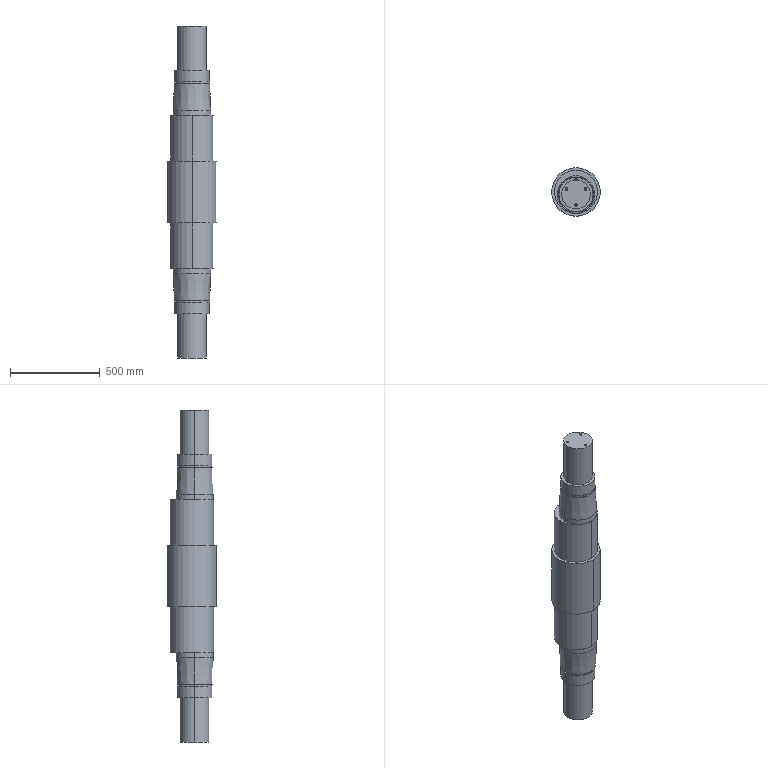Part | SolidWorks | features MirrorPattern 3, Revolution 2, 3DProfileFeature 1, CirPattern 1, HoleWzd 1, ICE 1 | 1 solid | 73 faces | box 270 x 270 x 1846 mm | volume 68110959 mm3 | cylinder 39 | plane 18 | cone 16 | commonest cylinder face diameters 14 x12 190 x6 160 x4 184 x4 208 x4 240 x4